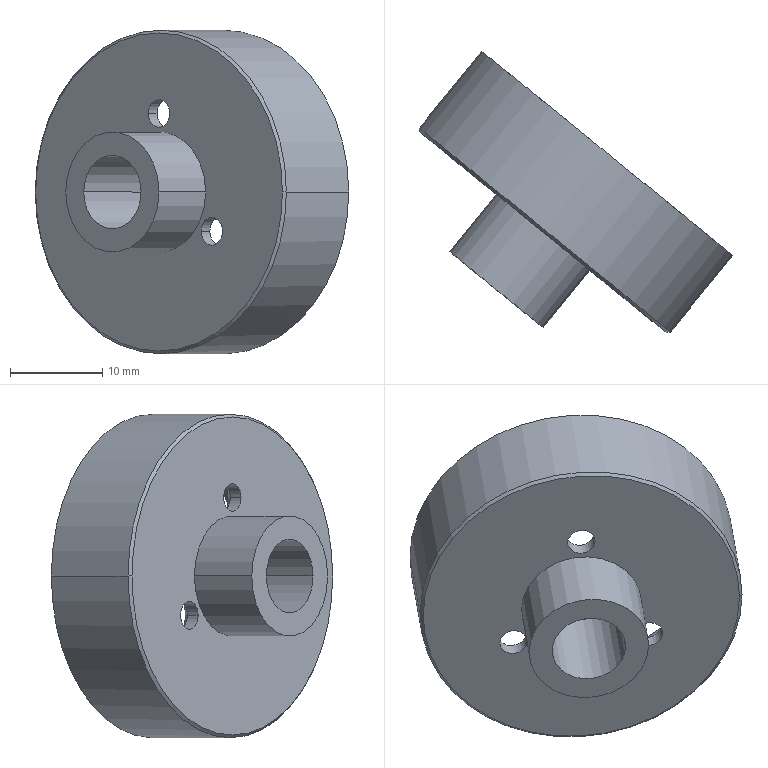Part | SolidWorks | features BaseBody 1 | 1 solid | 29 faces | box 33.905 x 30.428 x 35 mm | volume 5306 mm3 | cylinder 15 | cone 8 | plane 6 | commonest cylinder face diameters 3 x6 30 x3 8 x2 13 x2 35 x2
STEP:
#1=CARTESIAN_POINT('',(530.861,-127.065,299.195));
#2=VERTEX_POINT('',#1);
#3=CARTESIAN_POINT('',(557.55,-148.769,299.195));
#4=VERTEX_POINT('',#3);
#5=CARTESIAN_POINT('',(544.205,-137.917,299.195));
#6=DIRECTION('',(0.6309,0.7758,-0.000000012));
#7=DIRECTION('',(-0.7758,0.6309,0.));
#8=AXIS2_PLACEMENT_3D('',#5,#6,#7);
#9=CIRCLE('',#8,17.2);
#10=EDGE_CURVE('',#2,#4,#9,.T.);
#11=ORIENTED_EDGE('',*,*,#10,.T.);
#12=CARTESIAN_POINT('',(557.972,-148.726,299.195));
#13=VERTEX_POINT('',#12);
#14=CARTESIAN_POINT('',(557.972,-148.726,299.195));
#15=DIRECTION('',(0.9947,0.1025,-0.000000009));
#16=VECTOR('',#15,1000.);
#17=LINE('',#14,#16);
#18=EDGE_CURVE('',#4,#13,#17,.T.);
#19=ORIENTED_EDGE('',*,*,#18,.T.);
#20=CARTESIAN_POINT('',(530.818,-126.643,299.195));
#21=VERTEX_POINT('',#20);
#22=CARTESIAN_POINT('',(544.395,-137.684,299.195));
#23=DIRECTION('',(-0.6309,-0.7758,0.000000012));
#24=DIRECTION('',(-0.08545,0.06949,-0.9939));
#25=AXIS2_PLACEMENT_3D('',#22,#23,#24);
#26=CIRCLE('',#25,17.5);
#27=EDGE_CURVE('',#13,#21,#26,.T.);
#28=ORIENTED_EDGE('',*,*,#27,.T.);
#29=CARTESIAN_POINT('',(530.818,-126.643,299.195));
#30=DIRECTION('',(-0.1025,0.9947,-0.000000009));
#31=VECTOR('',#30,1000.);
#32=LINE('',#29,#31);
#33=EDGE_CURVE('',#2,#21,#32,.T.);
#34=ORIENTED_EDGE('',*,*,#33,.F.);
#35=EDGE_LOOP('',(#11,#19,#28,#34));
#36=FACE_OUTER_BOUND('',#35,.T.);
#37=CARTESIAN_POINT('',(544.395,-137.684,299.195));
#38=DIRECTION('',(0.6309,0.7758,-0.000000012));
#39=DIRECTION('',(-0.7758,0.6309,0.));
#40=AXIS2_PLACEMENT_3D('',#37,#38,#39);
#41=CONICAL_SURFACE('',#40,17.5,0.7854);
#42=ADVANCED_FACE('',(#36),#41,.T.);
#43=CARTESIAN_POINT('',(548.753,-141.615,294.945));
#44=VERTEX_POINT('',#43);
#45=CARTESIAN_POINT('',(551.08,-143.508,294.945));
#46=VERTEX_POINT('',#45);
#47=CARTESIAN_POINT('',(549.917,-142.562,294.945));
#48=DIRECTION('',(-0.6309,-0.7758,0.000000012));
#49=DIRECTION('',(-0.7758,0.6309,0.));
#50=AXIS2_PLACEMENT_3D('',#47,#48,#49);
#51=CIRCLE('',#50,1.5);
#52=EDGE_CURVE('',#44,#46,#51,.T.);
#53=ORIENTED_EDGE('',*,*,#52,.T.);
#54=CARTESIAN_POINT('',(552.027,-142.344,294.945));
#55=VERTEX_POINT('',#54);
#56=CARTESIAN_POINT('',(550.923,-143.702,294.945));
#57=DIRECTION('',(0.6309,0.7758,-0.000000012));
#58=VECTOR('',#57,1000.);
#59=LINE('',#56,#58);
#60=EDGE_CURVE('',#46,#55,#59,.T.);
#61=ORIENTED_EDGE('',*,*,#60,.T.);
#62=CARTESIAN_POINT('',(549.699,-140.451,294.945));
#63=VERTEX_POINT('',#62);
#64=CARTESIAN_POINT('',(550.863,-141.398,294.945));
#65=DIRECTION('',(-0.6309,-0.7758,0.000000012));
#66=DIRECTION('',(-0.7758,0.6309,0.));
#67=AXIS2_PLACEMENT_3D('',#64,#65,#66);
#68=CIRCLE('',#67,1.5);
#69=EDGE_CURVE('',#63,#55,#68,.T.);
#70=ORIENTED_EDGE('',*,*,#69,.F.);
#71=CARTESIAN_POINT('',(548.595,-141.809,294.945));
#72=DIRECTION('',(0.6309,0.7758,-0.000000012));
#73=VECTOR('',#72,1000.);
#74=LINE('',#71,#73);
#75=EDGE_CURVE('',#44,#63,#74,.T.);
#76=ORIENTED_EDGE('',*,*,#75,.F.);
#77=EDGE_LOOP('',(#53,#61,#70,#76));
#78=FACE_OUTER_BOUND('',#77,.T.);
#79=CARTESIAN_POINT('',(549.759,-142.756,294.945));
#80=DIRECTION('',(0.6309,0.7758,-0.000000012));
#81=DIRECTION('',(-0.7758,0.6309,0.));
#82=AXIS2_PLACEMENT_3D('',#79,#80,#81);
#83=CYLINDRICAL_SURFACE('',#82,1.5);
#84=ADVANCED_FACE('',(#78),#83,.F.);
#85=CARTESIAN_POINT('',(543.042,-136.971,307.695));
#86=VERTEX_POINT('',#85);
#87=CARTESIAN_POINT('',(545.369,-138.864,307.695));
#88=VERTEX_POINT('',#87);
#89=CARTESIAN_POINT('',(544.205,-137.917,307.695));
#90=DIRECTION('',(-0.6309,-0.7758,0.000000012));
#91=DIRECTION('',(-0.7758,0.6309,0.));
#92=AXIS2_PLACEMENT_3D('',#89,#90,#91);
#93=CIRCLE('',#92,1.5);
#94=EDGE_CURVE('',#86,#88,#93,.T.);
#95=ORIENTED_EDGE('',*,*,#94,.T.);
#96=CARTESIAN_POINT('',(546.316,-137.7,307.695));
#97=VERTEX_POINT('',#96);
#98=CARTESIAN_POINT('',(545.211,-139.058,307.695));
#99=DIRECTION('',(0.6309,0.7758,-0.000000012));
#100=VECTOR('',#99,1000.);
#101=LINE('',#98,#100);
#102=EDGE_CURVE('',#88,#97,#101,.T.);
#103=ORIENTED_EDGE('',*,*,#102,.T.);
#104=CARTESIAN_POINT('',(543.988,-135.807,307.695));
#105=VERTEX_POINT('',#104);
#106=CARTESIAN_POINT('',(545.152,-136.753,307.695));
#107=DIRECTION('',(-0.6309,-0.7758,0.000000012));
#108=DIRECTION('',(-0.7758,0.6309,0.));
#109=AXIS2_PLACEMENT_3D('',#106,#107,#108);
#110=CIRCLE('',#109,1.5);
#111=EDGE_CURVE('',#105,#97,#110,.T.);
#112=ORIENTED_EDGE('',*,*,#111,.F.);
#113=CARTESIAN_POINT('',(542.884,-137.165,307.695));
#114=DIRECTION('',(0.6309,0.7758,-0.000000012));
#115=VECTOR('',#114,1000.);
#116=LINE('',#113,#115);
#117=EDGE_CURVE('',#86,#105,#116,.T.);
#118=ORIENTED_EDGE('',*,*,#117,.F.);
#119=EDGE_LOOP('',(#95,#103,#112,#118));
#120=FACE_OUTER_BOUND('',#119,.T.);
#121=CARTESIAN_POINT('',(544.048,-138.111,307.695));
#122=DIRECTION('',(0.6309,0.7758,-0.000000012));
#123=DIRECTION('',(-0.7758,0.6309,0.));
#124=AXIS2_PLACEMENT_3D('',#121,#122,#123);
#125=CYLINDRICAL_SURFACE('',#124,1.5);
#126=ADVANCED_FACE('',(#120),#125,.F.);
#127=CARTESIAN_POINT('',(537.331,-132.326,294.945));
#128=VERTEX_POINT('',#127);
#129=CARTESIAN_POINT('',(539.658,-134.219,294.945));
#130=VERTEX_POINT('',#129);
#131=CARTESIAN_POINT('',(538.494,-133.273,294.945));
#132=DIRECTION('',(-0.6309,-0.7758,0.000000012));
#133=DIRECTION('',(-0.7758,0.6309,0.));
#134=AXIS2_PLACEMENT_3D('',#131,#132,#133);
#135=CIRCLE('',#134,1.5);
#136=EDGE_CURVE('',#128,#130,#135,.T.);
#137=ORIENTED_EDGE('',*,*,#136,.T.);
#138=CARTESIAN_POINT('',(540.604,-133.055,294.945));
#139=VERTEX_POINT('',#138);
#140=CARTESIAN_POINT('',(539.5,-134.413,294.945));
#141=DIRECTION('',(0.6309,0.7758,-0.000000012));
#142=VECTOR('',#141,1000.);
#143=LINE('',#140,#142);
#144=EDGE_CURVE('',#130,#139,#143,.T.);
#145=ORIENTED_EDGE('',*,*,#144,.T.);
#146=CARTESIAN_POINT('',(538.277,-131.163,294.945));
#147=VERTEX_POINT('',#146);
#148=CARTESIAN_POINT('',(539.441,-132.109,294.945));
#149=DIRECTION('',(-0.6309,-0.7758,0.000000012));
#150=DIRECTION('',(-0.7758,0.6309,0.));
#151=AXIS2_PLACEMENT_3D('',#148,#149,#150);
#152=CIRCLE('',#151,1.5);
#153=EDGE_CURVE('',#147,#139,#152,.T.);
#154=ORIENTED_EDGE('',*,*,#153,.F.);
#155=CARTESIAN_POINT('',(537.173,-132.52,294.945));
#156=DIRECTION('',(0.6309,0.7758,-0.000000012));
#157=VECTOR('',#156,1000.);
#158=LINE('',#155,#157);
#159=EDGE_CURVE('',#128,#147,#158,.T.);
#160=ORIENTED_EDGE('',*,*,#159,.F.);
#161=EDGE_LOOP('',(#137,#145,#154,#160));
#162=FACE_OUTER_BOUND('',#161,.T.);
#163=CARTESIAN_POINT('',(538.337,-133.467,294.945));
#164=DIRECTION('',(0.6309,0.7758,-0.000000012));
#165=DIRECTION('',(-0.7758,0.6309,0.));
#166=AXIS2_PLACEMENT_3D('',#163,#164,#165);
#167=CYLINDRICAL_SURFACE('',#166,1.5);
#168=ADVANCED_FACE('',(#162),#167,.F.);
#169=CARTESIAN_POINT('',(534.115,-140.023,299.195));
#170=VERTEX_POINT('',#169);
#171=CARTESIAN_POINT('',(544.201,-148.225,299.195));
#172=VERTEX_POINT('',#171);
#173=CARTESIAN_POINT('',(539.158,-144.124,299.195));
#174=DIRECTION('',(0.6309,0.7758,-0.000000012));
#175=DIRECTION('',(-0.7758,0.6309,0.));
#176=AXIS2_PLACEMENT_3D('',#173,#174,#175);
#177=CIRCLE('',#176,6.5);
#178=EDGE_CURVE('',#170,#172,#177,.T.);
#179=ORIENTED_EDGE('',*,*,#178,.T.);
#180=CARTESIAN_POINT('',(549.248,-142.018,299.195));
#181=VERTEX_POINT('',#180);
#182=CARTESIAN_POINT('',(549.248,-142.018,299.195));
#183=DIRECTION('',(0.6309,0.7758,-0.000000012));
#184=VECTOR('',#183,1000.);
#185=LINE('',#182,#184);
#186=EDGE_CURVE('',#172,#181,#185,.T.);
#187=ORIENTED_EDGE('',*,*,#186,.T.);
#188=CARTESIAN_POINT('',(539.162,-133.816,299.195));
#189=VERTEX_POINT('',#188);
#190=CARTESIAN_POINT('',(544.205,-137.917,299.195));
#191=DIRECTION('',(-0.6309,-0.7758,0.000000012));
#192=DIRECTION('',(-0.7758,0.6309,0.));
#193=AXIS2_PLACEMENT_3D('',#190,#191,#192);
#194=CIRCLE('',#193,6.5);
#195=EDGE_CURVE('',#181,#189,#194,.T.);
#196=ORIENTED_EDGE('',*,*,#195,.T.);
#197=CARTESIAN_POINT('',(539.162,-133.816,299.195));
#198=DIRECTION('',(0.6309,0.7758,-0.000000012));
#199=VECTOR('',#198,1000.);
#200=LINE('',#197,#199);
#201=EDGE_CURVE('',#170,#189,#200,.T.);
#202=ORIENTED_EDGE('',*,*,#201,.F.);
#203=EDGE_LOOP('',(#179,#187,#196,#202));
#204=FACE_OUTER_BOUND('',#203,.T.);
#205=CARTESIAN_POINT('',(544.205,-137.917,299.195));
#206=DIRECTION('',(0.6309,0.7758,-0.000000012));
#207=DIRECTION('',(-0.7758,0.6309,0.));
#208=AXIS2_PLACEMENT_3D('',#205,#206,#207);
#209=CYLINDRICAL_SURFACE('',#208,6.5);
#210=ADVANCED_FACE('',(#204),#209,.T.);
#211=CARTESIAN_POINT('',(564.723,-140.424,299.195));
#212=VERTEX_POINT('',#211);
#213=CARTESIAN_POINT('',(537.568,-118.342,299.195));
#214=VERTEX_POINT('',#213);
#215=CARTESIAN_POINT('',(551.146,-129.383,299.195));
#216=DIRECTION('',(-0.6309,-0.7758,0.000000012));
#217=DIRECTION('',(0.7758,-0.6309,0.));
#218=AXIS2_PLACEMENT_3D('',#215,#216,#217);
#219=CIRCLE('',#218,17.5);
#220=EDGE_CURVE('',#212,#214,#219,.T.);
#221=ORIENTED_EDGE('',*,*,#220,.T.);
#222=CARTESIAN_POINT('',(530.628,-126.876,299.195));
#223=DIRECTION('',(-0.6309,-0.7758,0.000000012));
#224=VECTOR('',#223,1000.);
#225=LINE('',#222,#224);
#226=EDGE_CURVE('',#214,#21,#225,.T.);
#227=ORIENTED_EDGE('',*,*,#226,.T.);
#228=ORIENTED_EDGE('',*,*,#27,.F.);
#229=CARTESIAN_POINT('',(557.783,-148.959,299.195));
#230=DIRECTION('',(-0.6309,-0.7758,0.000000012));
#231=VECTOR('',#230,1000.);
#232=LINE('',#229,#231);
#233=EDGE_CURVE('',#212,#13,#232,.T.);
#234=ORIENTED_EDGE('',*,*,#233,.F.);
#235=EDGE_LOOP('',(#221,#227,#228,#234));
#236=FACE_OUTER_BOUND('',#235,.T.);
#237=CARTESIAN_POINT('',(544.205,-137.917,299.195));
#238=DIRECTION('',(-0.6309,-0.7758,0.000000012));
#239=DIRECTION('',(0.7758,-0.6309,0.));
#240=AXIS2_PLACEMENT_3D('',#237,#238,#239);
#241=CYLINDRICAL_SURFACE('',#240,17.5);
#242=ADVANCED_FACE('',(#236),#241,.T.);
#243=ORIENTED_EDGE('',*,*,#69,.T.);
#244=CARTESIAN_POINT('',(554.137,-142.127,294.945));
#245=VERTEX_POINT('',#244);
#246=CARTESIAN_POINT('',(554.137,-142.127,294.945));
#247=DIRECTION('',(0.9947,0.1025,-0.000000009));
#248=VECTOR('',#247,1000.);
#249=LINE('',#246,#248);
#250=EDGE_CURVE('',#55,#245,#249,.T.);
#251=ORIENTED_EDGE('',*,*,#250,.T.);
#252=CARTESIAN_POINT('',(549.482,-138.341,294.945));
#253=VERTEX_POINT('',#252);
#254=CARTESIAN_POINT('',(551.809,-140.234,294.945));
#255=DIRECTION('',(-0.6309,-0.7758,0.000000012));
#256=DIRECTION('',(-0.7758,0.6309,0.));
#257=AXIS2_PLACEMENT_3D('',#254,#255,#256);
#258=CIRCLE('',#257,3.);
#259=EDGE_CURVE('',#253,#245,#258,.T.);
#260=ORIENTED_EDGE('',*,*,#259,.F.);
#261=CARTESIAN_POINT('',(549.482,-138.341,294.945));
#262=DIRECTION('',(-0.1025,0.9947,-0.000000009));
#263=VECTOR('',#262,1000.);
#264=LINE('',#261,#263);
#265=EDGE_CURVE('',#63,#253,#264,.T.);
#266=ORIENTED_EDGE('',*,*,#265,.F.);
#267=EDGE_LOOP('',(#243,#251,#260,#266));
#268=FACE_OUTER_BOUND('',#267,.T.);
#269=CARTESIAN_POINT('',(551.809,-140.234,294.945));
#270=DIRECTION('',(0.6309,0.7758,-0.000000012));
#271=DIRECTION('',(-0.7758,0.6309,0.));
#272=AXIS2_PLACEMENT_3D('',#269,#270,#271);
#273=CONICAL_SURFACE('',#272,3.,0.7854);
#274=ADVANCED_FACE('',(#268),#273,.F.);
#275=ORIENTED_EDGE('',*,*,#111,.T.);
#276=CARTESIAN_POINT('',(548.426,-137.483,307.695));
#277=VERTEX_POINT('',#276);
#278=CARTESIAN_POINT('',(548.426,-137.483,307.695));
#279=DIRECTION('',(0.9947,0.1025,-0.000000009));
#280=VECTOR('',#279,1000.);
#281=LINE('',#278,#280);
#282=EDGE_CURVE('',#97,#277,#281,.T.);
#283=ORIENTED_EDGE('',*,*,#282,.T.);
#284=CARTESIAN_POINT('',(543.771,-133.697,307.695));
#285=VERTEX_POINT('',#284);
#286=CARTESIAN_POINT('',(546.098,-135.59,307.695));
#287=DIRECTION('',(-0.6309,-0.7758,0.000000012));
#288=DIRECTION('',(-0.7758,0.6309,0.));
#289=AXIS2_PLACEMENT_3D('',#286,#287,#288);
#290=CIRCLE('',#289,3.);
#291=EDGE_CURVE('',#285,#277,#290,.T.);
#292=ORIENTED_EDGE('',*,*,#291,.F.);
#293=CARTESIAN_POINT('',(543.771,-133.697,307.695));
#294=DIRECTION('',(-0.1025,0.9947,-0.000000009));
#295=VECTOR('',#294,1000.);
#296=LINE('',#293,#295);
#297=EDGE_CURVE('',#105,#285,#296,.T.);
#298=ORIENTED_EDGE('',*,*,#297,.F.);
#299=EDGE_LOOP('',(#275,#283,#292,#298));
#300=FACE_OUTER_BOUND('',#299,.T.);
#301=CARTESIAN_POINT('',(546.098,-135.59,307.695));
#302=DIRECTION('',(0.6309,0.7758,-0.000000012));
#303=DIRECTION('',(-0.7758,0.6309,0.));
#304=AXIS2_PLACEMENT_3D('',#301,#302,#303);
#305=CONICAL_SURFACE('',#304,3.,0.7854);
#306=ADVANCED_FACE('',(#300),#305,.F.);
#307=ORIENTED_EDGE('',*,*,#153,.T.);
#308=CARTESIAN_POINT('',(542.715,-132.838,294.945));
#309=VERTEX_POINT('',#308);
#310=CARTESIAN_POINT('',(542.715,-132.838,294.945));
#311=DIRECTION('',(0.9947,0.1025,-0.000000009));
#312=VECTOR('',#311,1000.);
#313=LINE('',#310,#312);
#314=EDGE_CURVE('',#139,#309,#313,.T.);
#315=ORIENTED_EDGE('',*,*,#314,.T.);
#316=CARTESIAN_POINT('',(538.06,-129.053,294.945));
#317=VERTEX_POINT('',#316);
#318=CARTESIAN_POINT('',(540.387,-130.945,294.945));
#319=DIRECTION('',(-0.6309,-0.7758,0.000000012));
#320=DIRECTION('',(-0.7758,0.6309,0.));
#321=AXIS2_PLACEMENT_3D('',#318,#319,#320);
#322=CIRCLE('',#321,3.);
#323=EDGE_CURVE('',#317,#309,#322,.T.);
#324=ORIENTED_EDGE('',*,*,#323,.F.);
#325=CARTESIAN_POINT('',(538.06,-129.053,294.945));
#326=DIRECTION('',(-0.1025,0.9947,-0.000000009));
#327=VECTOR('',#326,1000.);
#328=LINE('',#325,#327);
#329=EDGE_CURVE('',#147,#317,#328,.T.);
#330=ORIENTED_EDGE('',*,*,#329,.F.);
#331=EDGE_LOOP('',(#307,#315,#324,#330));
#332=FACE_OUTER_BOUND('',#331,.T.);
#333=CARTESIAN_POINT('',(540.387,-130.945,294.945));
#334=DIRECTION('',(0.6309,0.7758,-0.000000012));
#335=DIRECTION('',(-0.7758,0.6309,0.));
#336=AXIS2_PLACEMENT_3D('',#333,#334,#335);
#337=CONICAL_SURFACE('',#336,3.,0.7854);
#338=ADVANCED_FACE('',(#332),#337,.F.);
#339=CARTESIAN_POINT('',(542.261,-146.648,299.195));
#340=VERTEX_POINT('',#339);
#341=CARTESIAN_POINT('',(536.055,-141.6,299.195));
#342=VERTEX_POINT('',#341);
#343=CARTESIAN_POINT('',(539.158,-144.124,299.195));
#344=DIRECTION('',(0.6309,0.7758,-0.000000012));
#345=DIRECTION('',(-0.7758,0.6309,0.));
#346=AXIS2_PLACEMENT_3D('',#343,#344,#345);
#347=CIRCLE('',#346,4.);
#348=EDGE_CURVE('',#340,#342,#347,.T.);
#349=ORIENTED_EDGE('',*,*,#348,.F.);
#350=CARTESIAN_POINT('',(549.202,-138.113,299.195));
#351=VERTEX_POINT('',#350);
#352=CARTESIAN_POINT('',(549.202,-138.113,299.195));
#353=DIRECTION('',(0.6309,0.7758,-0.000000012));
#354=VECTOR('',#353,1000.);
#355=LINE('',#352,#354);
#356=EDGE_CURVE('',#340,#351,#355,.T.);
#357=ORIENTED_EDGE('',*,*,#356,.T.);
#358=CARTESIAN_POINT('',(542.995,-133.066,299.195));
#359=VERTEX_POINT('',#358);
#360=CARTESIAN_POINT('',(546.098,-135.59,299.195));
#361=DIRECTION('',(0.6309,0.7758,-0.000000012));
#362=DIRECTION('',(-0.7758,0.6309,0.));
#363=AXIS2_PLACEMENT_3D('',#360,#361,#362);
#364=CIRCLE('',#363,4.);
#365=EDGE_CURVE('',#351,#359,#364,.T.);
#366=ORIENTED_EDGE('',*,*,#365,.T.);
#367=CARTESIAN_POINT('',(542.995,-133.066,299.195));
#368=DIRECTION('',(0.6309,0.7758,-0.000000012));
#369=VECTOR('',#368,1000.);
#370=LINE('',#367,#369);
#371=EDGE_CURVE('',#342,#359,#370,.T.);
#372=ORIENTED_EDGE('',*,*,#371,.F.);
#373=EDGE_LOOP('',(#349,#357,#366,#372));
#374=FACE_OUTER_BOUND('',#373,.T.);
#375=CARTESIAN_POINT('',(546.098,-135.59,299.195));
#376=DIRECTION('',(0.6309,0.7758,-0.000000012));
#377=DIRECTION('',(-0.7758,0.6309,0.));
#378=AXIS2_PLACEMENT_3D('',#375,#376,#377);
#379=CYLINDRICAL_SURFACE('',#378,4.);
#380=ADVANCED_FACE('',(#374),#379,.F.);
#381=CARTESIAN_POINT('',(539.508,-119.919,299.195));
#382=VERTEX_POINT('',#381);
#383=CARTESIAN_POINT('',(550.755,-129.066,284.203));
#384=VERTEX_POINT('',#383);
#385=CARTESIAN_POINT('',(551.146,-129.383,299.195));
#386=DIRECTION('',(-0.6309,-0.7758,0.000000012));
#387=DIRECTION('',(0.7758,-0.6309,0.));
#388=AXIS2_PLACEMENT_3D('',#385,#386,#387);
#389=CIRCLE('',#388,15.);
#390=EDGE_CURVE('',#382,#384,#389,.T.);
#391=ORIENTED_EDGE('',*,*,#390,.F.);
#392=CARTESIAN_POINT('',(534.461,-126.126,299.195));
#393=VERTEX_POINT('',#392);
#394=CARTESIAN_POINT('',(539.508,-119.919,299.195));
#395=DIRECTION('',(-0.6309,-0.7758,0.000000012));
#396=VECTOR('',#395,1000.);
#397=LINE('',#394,#396);
#398=EDGE_CURVE('',#382,#393,#397,.T.);
#399=ORIENTED_EDGE('',*,*,#398,.T.);
#400=CARTESIAN_POINT('',(545.708,-135.272,284.203));
#401=VERTEX_POINT('',#400);
#402=CARTESIAN_POINT('',(546.098,-135.59,299.195));
#403=DIRECTION('',(-0.6309,-0.7758,0.000000012));
#404=DIRECTION('',(0.7758,-0.6309,0.));
#405=AXIS2_PLACEMENT_3D('',#402,#403,#404);
#406=CIRCLE('',#405,15.);
#407=EDGE_CURVE('',#393,#401,#406,.T.);
#408=ORIENTED_EDGE('',*,*,#407,.T.);
#409=CARTESIAN_POINT('',(550.755,-129.066,284.203));
#410=DIRECTION('',(0.6309,0.7758,0.));
#411=VECTOR('',#410,1000.);
#412=LINE('',#409,#411);
#413=EDGE_CURVE('',#401,#384,#412,.T.);
#414=ORIENTED_EDGE('',*,*,#413,.T.);
#415=EDGE_LOOP('',(#391,#399,#408,#414));
#416=FACE_OUTER_BOUND('',#415,.T.);
#417=CARTESIAN_POINT('',(551.146,-129.383,299.195));
#418=DIRECTION('',(-0.6309,-0.7758,0.000000012));
#419=DIRECTION('',(0.7758,-0.6309,0.));
#420=AXIS2_PLACEMENT_3D('',#417,#418,#419);
#421=CYLINDRICAL_SURFACE('',#420,15.);
#422=ADVANCED_FACE('',(#416),#421,.F.);
#423=ORIENTED_EDGE('',*,*,#398,.F.);
#424=CARTESIAN_POINT('',(562.783,-138.847,299.195));
#425=VERTEX_POINT('',#424);
#426=CARTESIAN_POINT('',(551.146,-129.383,299.195));
#427=DIRECTION('',(-0.6309,-0.7758,0.000000012));
#428=DIRECTION('',(0.7758,-0.6309,0.));
#429=AXIS2_PLACEMENT_3D('',#426,#427,#428);
#430=CIRCLE('',#429,15.);
#431=EDGE_CURVE('',#425,#382,#430,.T.);
#432=ORIENTED_EDGE('',*,*,#431,.F.);
#433=CARTESIAN_POINT('',(557.736,-145.054,299.195));
#434=VERTEX_POINT('',#433);
#435=CARTESIAN_POINT('',(562.783,-138.847,299.195));
#436=DIRECTION('',(-0.6309,-0.7758,0.000000012));
#437=VECTOR('',#436,1000.);
#438=LINE('',#435,#437);
#439=EDGE_CURVE('',#425,#434,#438,.T.);
#440=ORIENTED_EDGE('',*,*,#439,.T.);
#441=CARTESIAN_POINT('',(546.098,-135.59,299.195));
#442=DIRECTION('',(-0.6309,-0.7758,0.000000012));
#443=DIRECTION('',(0.7758,-0.6309,0.));
#444=AXIS2_PLACEMENT_3D('',#441,#442,#443);
#445=CIRCLE('',#444,15.);
#446=EDGE_CURVE('',#434,#393,#445,.T.);
#447=ORIENTED_EDGE('',*,*,#446,.T.);
#448=EDGE_LOOP('',(#423,#432,#440,#447));
#449=FACE_OUTER_BOUND('',#448,.T.);
#450=CARTESIAN_POINT('',(551.146,-129.383,299.195));
#451=DIRECTION('',(-0.6309,-0.7758,0.000000012));
#452=DIRECTION('',(0.7758,-0.6309,0.));
#453=AXIS2_PLACEMENT_3D('',#450,#451,#452);
#454=CYLINDRICAL_SURFACE('',#453,15.);
#455=ADVANCED_FACE('',(#449),#454,.F.);
#456=ORIENTED_EDGE('',*,*,#10,.F.);
#457=CARTESIAN_POINT('',(544.205,-137.917,299.195));
#458=DIRECTION('',(0.6309,0.7758,-0.000000012));
#459=DIRECTION('',(-0.7758,0.6309,0.));
#460=AXIS2_PLACEMENT_3D('',#457,#458,#459);
#461=CIRCLE('',#460,17.2);
#462=EDGE_CURVE('',#4,#2,#461,.T.);
#463=ORIENTED_EDGE('',*,*,#462,.F.);
#464=EDGE_LOOP('',(#456,#463));
#465=FACE_OUTER_BOUND('',#464,.T.);
#466=ORIENTED_EDGE('',*,*,#52,.F.);
#467=CARTESIAN_POINT('',(549.917,-142.562,294.945));
#468=DIRECTION('',(-0.6309,-0.7758,0.000000012));
#469=DIRECTION('',(-0.7758,0.6309,0.));
#470=AXIS2_PLACEMENT_3D('',#467,#468,#469);
#471=CIRCLE('',#470,1.5);
#472=EDGE_CURVE('',#46,#44,#471,.T.);
#473=ORIENTED_EDGE('',*,*,#472,.F.);
#474=EDGE_LOOP('',(#466,#473));
#475=FACE_BOUND('',#474,.T.);
#476=ORIENTED_EDGE('',*,*,#94,.F.);
#477=CARTESIAN_POINT('',(544.205,-137.917,307.695));
#478=DIRECTION('',(-0.6309,-0.7758,0.000000012));
#479=DIRECTION('',(-0.7758,0.6309,0.));
#480=AXIS2_PLACEMENT_3D('',#477,#478,#479);
#481=CIRCLE('',#480,1.5);
#482=EDGE_CURVE('',#88,#86,#481,.T.);
#483=ORIENTED_EDGE('',*,*,#482,.F.);
#484=EDGE_LOOP('',(#476,#483));
#485=FACE_BOUND('',#484,.T.);
#486=ORIENTED_EDGE('',*,*,#136,.F.);
#487=CARTESIAN_POINT('',(538.494,-133.273,294.945));
#488=DIRECTION('',(-0.6309,-0.7758,0.000000012));
#489=DIRECTION('',(-0.7758,0.6309,0.));
#490=AXIS2_PLACEMENT_3D('',#487,#488,#489);
#491=CIRCLE('',#490,1.5);
#492=EDGE_CURVE('',#130,#128,#491,.T.);
#493=ORIENTED_EDGE('',*,*,#492,.F.);
#494=EDGE_LOOP('',(#486,#493));
#495=FACE_BOUND('',#494,.T.);
#496=CARTESIAN_POINT('',(544.205,-137.917,299.195));
#497=DIRECTION('',(-0.6309,-0.7758,0.000000012));
#498=DIRECTION('',(-0.7758,0.6309,0.));
#499=AXIS2_PLACEMENT_3D('',#496,#497,#498);
#500=CIRCLE('',#499,6.5);
#501=EDGE_CURVE('',#189,#181,#500,.T.);
#502=ORIENTED_EDGE('',*,*,#501,.F.);
#503=ORIENTED_EDGE('',*,*,#195,.F.);
#504=EDGE_LOOP('',(#502,#503));
#505=FACE_BOUND('',#504,.T.);
#506=CARTESIAN_POINT('',(544.205,-137.917,299.195));
#507=DIRECTION('',(0.6309,0.7758,-0.000000012));
#508=DIRECTION('',(-0.7758,0.6309,0.));
#509=AXIS2_PLACEMENT_3D('',#506,#507,#508);
#510=PLANE('',#509);
#511=ADVANCED_FACE('',(#465,#475,#485,#495,#505),#510,.F.);
#512=ORIENTED_EDGE('',*,*,#18,.F.);
#513=ORIENTED_EDGE('',*,*,#462,.T.);
#514=ORIENTED_EDGE('',*,*,#33,.T.);
#515=CARTESIAN_POINT('',(544.395,-137.684,299.195));
#516=DIRECTION('',(-0.6309,-0.7758,0.000000012));
#517=DIRECTION('',(-0.08545,0.06949,-0.9939));
#518=AXIS2_PLACEMENT_3D('',#515,#516,#517);
#519=CIRCLE('',#518,17.5);
#520=EDGE_CURVE('',#21,#13,#519,.T.);
#521=ORIENTED_EDGE('',*,*,#520,.T.);
#522=EDGE_LOOP('',(#512,#513,#514,#521));
#523=FACE_OUTER_BOUND('',#522,.T.);
#524=CARTESIAN_POINT('',(544.395,-137.684,299.195));
#525=DIRECTION('',(0.6309,0.7758,-0.000000012));
#526=DIRECTION('',(-0.7758,0.6309,0.));
#527=AXIS2_PLACEMENT_3D('',#524,#525,#526);
#528=CONICAL_SURFACE('',#527,17.5,0.7854);
#529=ADVANCED_FACE('',(#523),#528,.T.);
#530=ORIENTED_EDGE('',*,*,#60,.F.);
#531=ORIENTED_EDGE('',*,*,#472,.T.);
#532=ORIENTED_EDGE('',*,*,#75,.T.);
#533=CARTESIAN_POINT('',(550.863,-141.398,294.945));
#534=DIRECTION('',(-0.6309,-0.7758,0.000000012));
#535=DIRECTION('',(-0.7758,0.6309,0.));
#536=AXIS2_PLACEMENT_3D('',#533,#534,#535);
#537=CIRCLE('',#536,1.5);
#538=EDGE_CURVE('',#55,#63,#537,.T.);
#539=ORIENTED_EDGE('',*,*,#538,.F.);
#540=EDGE_LOOP('',(#530,#531,#532,#539));
#541=FACE_OUTER_BOUND('',#540,.T.);
#542=CARTESIAN_POINT('',(549.759,-142.756,294.945));
#543=DIRECTION('',(0.6309,0.7758,-0.000000012));
#544=DIRECTION('',(-0.7758,0.6309,0.));
#545=AXIS2_PLACEMENT_3D('',#542,#543,#544);
#546=CYLINDRICAL_SURFACE('',#545,1.5);
#547=ADVANCED_FACE('',(#541),#546,.F.);
#548=ORIENTED_EDGE('',*,*,#102,.F.);
#549=ORIENTED_EDGE('',*,*,#482,.T.);
#550=ORIENTED_EDGE('',*,*,#117,.T.);
#551=CARTESIAN_POINT('',(545.152,-136.753,307.695));
#552=DIRECTION('',(-0.6309,-0.7758,0.000000012));
#553=DIRECTION('',(-0.7758,0.6309,0.));
#554=AXIS2_PLACEMENT_3D('',#551,#552,#553);
#555=CIRCLE('',#554,1.5);
#556=EDGE_CURVE('',#97,#105,#555,.T.);
#557=ORIENTED_EDGE('',*,*,#556,.F.);
#558=EDGE_LOOP('',(#548,#549,#550,#557));
#559=FACE_OUTER_BOUND('',#558,.T.);
#560=CARTESIAN_POINT('',(544.048,-138.111,307.695));
#561=DIRECTION('',(0.6309,0.7758,-0.000000012));
#562=DIRECTION('',(-0.7758,0.6309,0.));
#563=AXIS2_PLACEMENT_3D('',#560,#561,#562);
#564=CYLINDRICAL_SURFACE('',#563,1.5);
#565=ADVANCED_FACE('',(#559),#564,.F.);
#566=ORIENTED_EDGE('',*,*,#144,.F.);
#567=ORIENTED_EDGE('',*,*,#492,.T.);
#568=ORIENTED_EDGE('',*,*,#159,.T.);
#569=CARTESIAN_POINT('',(539.441,-132.109,294.945));
#570=DIRECTION('',(-0.6309,-0.7758,0.000000012));
#571=DIRECTION('',(-0.7758,0.6309,0.));
#572=AXIS2_PLACEMENT_3D('',#569,#570,#571);
#573=CIRCLE('',#572,1.5);
#574=EDGE_CURVE('',#139,#147,#573,.T.);
#575=ORIENTED_EDGE('',*,*,#574,.F.);
#576=EDGE_LOOP('',(#566,#567,#568,#575));
#577=FACE_OUTER_BOUND('',#576,.T.);
#578=CARTESIAN_POINT('',(538.337,-133.467,294.945));
#579=DIRECTION('',(0.6309,0.7758,-0.000000012));
#580=DIRECTION('',(-0.7758,0.6309,0.));
#581=AXIS2_PLACEMENT_3D('',#578,#579,#580);
#582=CYLINDRICAL_SURFACE('',#581,1.5);
#583=ADVANCED_FACE('',(#577),#582,.F.);
#584=ORIENTED_EDGE('',*,*,#186,.F.);
#585=CARTESIAN_POINT('',(539.158,-144.124,299.195));
#586=DIRECTION('',(0.6309,0.7758,-0.000000012));
#587=DIRECTION('',(-0.7758,0.6309,0.));
#588=AXIS2_PLACEMENT_3D('',#585,#586,#587);
#589=CIRCLE('',#588,6.5);
#590=EDGE_CURVE('',#172,#170,#589,.T.);
#591=ORIENTED_EDGE('',*,*,#590,.T.);
#592=ORIENTED_EDGE('',*,*,#201,.T.);
#593=ORIENTED_EDGE('',*,*,#501,.T.);
#594=EDGE_LOOP('',(#584,#591,#592,#593));
#595=FACE_OUTER_BOUND('',#594,.T.);
#596=CARTESIAN_POINT('',(544.205,-137.917,299.195));
#597=DIRECTION('',(0.6309,0.7758,-0.000000012));
#598=DIRECTION('',(-0.7758,0.6309,0.));
#599=AXIS2_PLACEMENT_3D('',#596,#597,#598);
#600=CYLINDRICAL_SURFACE('',#599,6.5);
#601=ADVANCED_FACE('',(#595),#600,.T.);
#602=ORIENTED_EDGE('',*,*,#226,.F.);
#603=CARTESIAN_POINT('',(550.755,-129.066,281.702));
#604=VERTEX_POINT('',#603);
#605=CARTESIAN_POINT('',(551.146,-129.383,299.195));
#606=DIRECTION('',(-0.6309,-0.7758,0.000000012));
#607=DIRECTION('',(0.7758,-0.6309,0.));
#608=AXIS2_PLACEMENT_3D('',#605,#606,#607);
#609=CIRCLE('',#608,17.5);
#610=EDGE_CURVE('',#214,#604,#609,.T.);
#611=ORIENTED_EDGE('',*,*,#610,.T.);
#612=CARTESIAN_POINT('',(545.708,-135.272,281.702));
#613=VERTEX_POINT('',#612);
#614=CARTESIAN_POINT('',(543.815,-137.6,281.702));
#615=DIRECTION('',(-0.6309,-0.7758,0.000000012));
#616=VECTOR('',#615,1000.);
#617=LINE('',#614,#616);
#618=EDGE_CURVE('',#604,#613,#617,.T.);
#619=ORIENTED_EDGE('',*,*,#618,.T.);
#620=CARTESIAN_POINT('',(546.484,-135.903,281.702));
#621=VERTEX_POINT('',#620);
#622=CARTESIAN_POINT('',(546.098,-135.59,299.195));
#623=DIRECTION('',(-0.6309,-0.7758,0.000000012));
#624=DIRECTION('',(0.7758,-0.6309,0.));
#625=AXIS2_PLACEMENT_3D('',#622,#623,#624);
#626=CIRCLE('',#625,17.5);
#627=EDGE_CURVE('',#613,#621,#626,.T.);
#628=ORIENTED_EDGE('',*,*,#627,.T.);
#629=CARTESIAN_POINT('',(551.531,-129.697,281.702));
#630=VERTEX_POINT('',#629);
#631=CARTESIAN_POINT('',(544.591,-138.231,281.702));
#632=DIRECTION('',(0.6309,0.7758,-0.000000012));
#633=VECTOR('',#632,1000.);
#634=LINE('',#631,#633);
#635=EDGE_CURVE('',#621,#630,#634,.T.);
#636=ORIENTED_EDGE('',*,*,#635,.T.);
#637=CARTESIAN_POINT('',(551.146,-129.383,299.195));
#638=DIRECTION('',(-0.6309,-0.7758,0.000000012));
#639=DIRECTION('',(0.7758,-0.6309,0.));
#640=AXIS2_PLACEMENT_3D('',#637,#638,#639);
#641=CIRCLE('',#640,17.5);
#642=EDGE_CURVE('',#630,#212,#641,.T.);
#643=ORIENTED_EDGE('',*,*,#642,.T.);
#644=ORIENTED_EDGE('',*,*,#233,.T.);
#645=ORIENTED_EDGE('',*,*,#520,.F.);
#646=EDGE_LOOP('',(#602,#611,#619,#628,#636,#643,#644,#645));
#647=FACE_OUTER_BOUND('',#646,.T.);
#648=CARTESIAN_POINT('',(544.205,-137.917,299.195));
#649=DIRECTION('',(-0.6309,-0.7758,0.000000012));
#650=DIRECTION('',(0.7758,-0.6309,0.));
#651=AXIS2_PLACEMENT_3D('',#648,#649,#650);
#652=CYLINDRICAL_SURFACE('',#651,17.5);
#653=ADVANCED_FACE('',(#647),#652,.T.);
#654=ORIENTED_EDGE('',*,*,#250,.F.);
#655=ORIENTED_EDGE('',*,*,#538,.T.);
#656=ORIENTED_EDGE('',*,*,#265,.T.);
#657=CARTESIAN_POINT('',(551.809,-140.234,294.945));
#658=DIRECTION('',(-0.6309,-0.7758,0.000000012));
#659=DIRECTION('',(-0.7758,0.6309,0.));
#660=AXIS2_PLACEMENT_3D('',#657,#658,#659);
#661=CIRCLE('',#660,3.);
#662=EDGE_CURVE('',#245,#253,#661,.T.);
#663=ORIENTED_EDGE('',*,*,#662,.F.);
#664=EDGE_LOOP('',(#654,#655,#656,#663));
#665=FACE_OUTER_BOUND('',#664,.T.);
#666=CARTESIAN_POINT('',(551.809,-140.234,294.945));
#667=DIRECTION('',(0.6309,0.7758,-0.000000012));
#668=DIRECTION('',(-0.7758,0.6309,0.));
#669=AXIS2_PLACEMENT_3D('',#666,#667,#668);
#670=CONICAL_SURFACE('',#669,3.,0.7854);
#671=ADVANCED_FACE('',(#665),#670,.F.);
#672=ORIENTED_EDGE('',*,*,#282,.F.);
#673=ORIENTED_EDGE('',*,*,#556,.T.);
#674=ORIENTED_EDGE('',*,*,#297,.T.);
#675=CARTESIAN_POINT('',(546.098,-135.59,307.695));
#676=DIRECTION('',(-0.6309,-0.7758,0.000000012));
#677=DIRECTION('',(-0.7758,0.6309,0.));
#678=AXIS2_PLACEMENT_3D('',#675,#676,#677);
#679=CIRCLE('',#678,3.);
#680=EDGE_CURVE('',#277,#285,#679,.T.);
#681=ORIENTED_EDGE('',*,*,#680,.F.);
#682=EDGE_LOOP('',(#672,#673,#674,#681));
#683=FACE_OUTER_BOUND('',#682,.T.);
#684=CARTESIAN_POINT('',(546.098,-135.59,307.695));
#685=DIRECTION('',(0.6309,0.7758,-0.000000012));
#686=DIRECTION('',(-0.7758,0.6309,0.));
#687=AXIS2_PLACEMENT_3D('',#684,#685,#686);
#688=CONICAL_SURFACE('',#687,3.,0.7854);
#689=ADVANCED_FACE('',(#683),#688,.F.);
#690=ORIENTED_EDGE('',*,*,#314,.F.);
#691=ORIENTED_EDGE('',*,*,#574,.T.);
#692=ORIENTED_EDGE('',*,*,#329,.T.);
#693=CARTESIAN_POINT('',(540.387,-130.945,294.945));
#694=DIRECTION('',(-0.6309,-0.7758,0.000000012));
#695=DIRECTION('',(-0.7758,0.6309,0.));
#696=AXIS2_PLACEMENT_3D('',#693,#694,#695);
#697=CIRCLE('',#696,3.);
#698=EDGE_CURVE('',#309,#317,#697,.T.);
#699=ORIENTED_EDGE('',*,*,#698,.F.);
#700=EDGE_LOOP('',(#690,#691,#692,#699));
#701=FACE_OUTER_BOUND('',#700,.T.);
#702=CARTESIAN_POINT('',(540.387,-130.945,294.945));
#703=DIRECTION('',(0.6309,0.7758,-0.000000012));
#704=DIRECTION('',(-0.7758,0.6309,0.));
#705=AXIS2_PLACEMENT_3D('',#702,#703,#704);
#706=CONICAL_SURFACE('',#705,3.,0.7854);
#707=ADVANCED_FACE('',(#701),#706,.F.);
#708=ORIENTED_EDGE('',*,*,#178,.F.);
#709=ORIENTED_EDGE('',*,*,#590,.F.);
#710=EDGE_LOOP('',(#708,#709));
#711=FACE_OUTER_BOUND('',#710,.T.);
#712=CARTESIAN_POINT('',(539.158,-144.124,299.195));
#713=DIRECTION('',(0.6309,0.7758,-0.000000012));
#714=DIRECTION('',(-0.7758,0.6309,0.));
#715=AXIS2_PLACEMENT_3D('',#712,#713,#714);
#716=CIRCLE('',#715,4.);
#717=EDGE_CURVE('',#342,#340,#716,.T.);
#718=ORIENTED_EDGE('',*,*,#717,.T.);
#719=ORIENTED_EDGE('',*,*,#348,.T.);
#720=EDGE_LOOP('',(#718,#719));
#721=FACE_BOUND('',#720,.T.);
#722=CARTESIAN_POINT('',(539.158,-144.124,299.195));
#723=DIRECTION('',(-0.6309,-0.7758,0.000000012));
#724=DIRECTION('',(0.7758,-0.6309,0.));
#725=AXIS2_PLACEMENT_3D('',#722,#723,#724);
#726=PLANE('',#725);
#727=ADVANCED_FACE('',(#711,#721),#726,.T.);
#728=CARTESIAN_POINT('',(551.531,-129.697,284.203));
#729=VERTEX_POINT('',#728);
#730=CARTESIAN_POINT('',(551.146,-129.383,299.195));
#731=DIRECTION('',(-0.6309,-0.7758,0.000000012));
#732=DIRECTION('',(0.7758,-0.6309,0.));
#733=AXIS2_PLACEMENT_3D('',#730,#731,#732);
#734=CIRCLE('',#733,15.);
#735=EDGE_CURVE('',#729,#425,#734,.T.);
#736=ORIENTED_EDGE('',*,*,#735,.T.);
#737=ORIENTED_EDGE('',*,*,#431,.T.);
#738=ORIENTED_EDGE('',*,*,#390,.T.);
#739=CARTESIAN_POINT('',(550.755,-129.066,299.195));
#740=DIRECTION('',(-0.000000008,-0.000000009,-1.));
#741=VECTOR('',#740,1000.);
#742=LINE('',#739,#741);
#743=EDGE_CURVE('',#384,#604,#742,.T.);
#744=ORIENTED_EDGE('',*,*,#743,.T.);
#745=ORIENTED_EDGE('',*,*,#610,.F.);
#746=ORIENTED_EDGE('',*,*,#220,.F.);
#747=ORIENTED_EDGE('',*,*,#642,.F.);
#748=CARTESIAN_POINT('',(551.531,-129.697,299.195));
#749=DIRECTION('',(0.000000008,0.000000009,1.));
#750=VECTOR('',#749,1000.);
#751=LINE('',#748,#750);
#752=EDGE_CURVE('',#630,#729,#751,.T.);
#753=ORIENTED_EDGE('',*,*,#752,.T.);
#754=EDGE_LOOP('',(#736,#737,#738,#744,#745,#746,#747,#753));
#755=FACE_OUTER_BOUND('',#754,.T.);
#756=CARTESIAN_POINT('',(551.146,-129.383,299.195));
#757=DIRECTION('',(0.6309,0.7758,-0.000000012));
#758=DIRECTION('',(-0.7758,0.6309,0.));
#759=AXIS2_PLACEMENT_3D('',#756,#757,#758);
#760=PLANE('',#759);
#761=ADVANCED_FACE('',(#755),#760,.T.);
#762=ORIENTED_EDGE('',*,*,#752,.F.);
#763=ORIENTED_EDGE('',*,*,#635,.F.);
#764=CARTESIAN_POINT('',(546.484,-135.903,284.203));
#765=VERTEX_POINT('',#764);
#766=CARTESIAN_POINT('',(546.484,-135.903,287.719));
#767=DIRECTION('',(-0.000000016,0.000000013,-1.));
#768=VECTOR('',#767,1000.);
#769=LINE('',#766,#768);
#770=EDGE_CURVE('',#765,#621,#769,.T.);
#771=ORIENTED_EDGE('',*,*,#770,.F.);
#772=CARTESIAN_POINT('',(551.531,-129.697,284.203));
#773=DIRECTION('',(-0.6309,-0.7758,0.));
#774=VECTOR('',#773,1000.);
#775=LINE('',#772,#774);
#776=EDGE_CURVE('',#729,#765,#775,.T.);
#777=ORIENTED_EDGE('',*,*,#776,.F.);
#778=EDGE_LOOP('',(#762,#763,#771,#777));
#779=FACE_OUTER_BOUND('',#778,.T.);
#780=CARTESIAN_POINT('',(551.531,-129.697,287.719));
#781=DIRECTION('',(0.7758,-0.6309,-0.000000021));
#782=DIRECTION('',(0.6309,0.7758,0.));
#783=AXIS2_PLACEMENT_3D('',#780,#781,#782);
#784=PLANE('',#783);
#785=ADVANCED_FACE('',(#779),#784,.F.);
#786=CARTESIAN_POINT('',(545.708,-135.272,279.776));
#787=DIRECTION('',(0.000000016,-0.000000013,1.));
#788=VECTOR('',#787,1000.);
#789=LINE('',#786,#788);
#790=EDGE_CURVE('',#613,#401,#789,.T.);
#791=ORIENTED_EDGE('',*,*,#790,.F.);
#792=ORIENTED_EDGE('',*,*,#618,.F.);
#793=ORIENTED_EDGE('',*,*,#743,.F.);
#794=ORIENTED_EDGE('',*,*,#413,.F.);
#795=EDGE_LOOP('',(#791,#792,#793,#794));
#796=FACE_OUTER_BOUND('',#795,.T.);
#797=CARTESIAN_POINT('',(550.755,-129.066,279.776));
#798=DIRECTION('',(-0.7758,0.6309,0.000000021));
#799=DIRECTION('',(-0.6309,-0.7758,0.));
#800=AXIS2_PLACEMENT_3D('',#797,#798,#799);
#801=PLANE('',#800);
#802=ADVANCED_FACE('',(#796),#801,.F.);
#803=CARTESIAN_POINT('',(546.098,-135.59,299.195));
#804=DIRECTION('',(-0.6309,-0.7758,0.000000012));
#805=DIRECTION('',(0.7758,-0.6309,0.));
#806=AXIS2_PLACEMENT_3D('',#803,#804,#805);
#807=CIRCLE('',#806,15.);
#808=EDGE_CURVE('',#765,#434,#807,.T.);
#809=ORIENTED_EDGE('',*,*,#808,.F.);
#810=ORIENTED_EDGE('',*,*,#770,.T.);
#811=ORIENTED_EDGE('',*,*,#627,.F.);
#812=ORIENTED_EDGE('',*,*,#790,.T.);
#813=ORIENTED_EDGE('',*,*,#407,.F.);
#814=ORIENTED_EDGE('',*,*,#446,.F.);
#815=EDGE_LOOP('',(#809,#810,#811,#812,#813,#814));
#816=FACE_OUTER_BOUND('',#815,.T.);
#817=ORIENTED_EDGE('',*,*,#259,.T.);
#818=ORIENTED_EDGE('',*,*,#662,.T.);
#819=EDGE_LOOP('',(#817,#818));
#820=FACE_BOUND('',#819,.T.);
#821=ORIENTED_EDGE('',*,*,#291,.T.);
#822=ORIENTED_EDGE('',*,*,#680,.T.);
#823=EDGE_LOOP('',(#821,#822));
#824=FACE_BOUND('',#823,.T.);
#825=ORIENTED_EDGE('',*,*,#323,.T.);
#826=ORIENTED_EDGE('',*,*,#698,.T.);
#827=EDGE_LOOP('',(#825,#826));
#828=FACE_BOUND('',#827,.T.);
#829=CARTESIAN_POINT('',(546.098,-135.59,299.195));
#830=DIRECTION('',(0.6309,0.7758,-0.000000012));
#831=DIRECTION('',(-0.7758,0.6309,0.));
#832=AXIS2_PLACEMENT_3D('',#829,#830,#831);
#833=CIRCLE('',#832,4.);
#834=EDGE_CURVE('',#359,#351,#833,.T.);
#835=ORIENTED_EDGE('',*,*,#834,.F.);
#836=ORIENTED_EDGE('',*,*,#365,.F.);
#837=EDGE_LOOP('',(#835,#836));
#838=FACE_BOUND('',#837,.T.);
#839=CARTESIAN_POINT('',(546.098,-135.59,299.195));
#840=DIRECTION('',(-0.6309,-0.7758,0.000000012));
#841=DIRECTION('',(0.7758,-0.6309,0.));
#842=AXIS2_PLACEMENT_3D('',#839,#840,#841);
#843=PLANE('',#842);
#844=ADVANCED_FACE('',(#816,#820,#824,#828,#838),#843,.F.);
#845=ORIENTED_EDGE('',*,*,#356,.F.);
#846=ORIENTED_EDGE('',*,*,#717,.F.);
#847=ORIENTED_EDGE('',*,*,#371,.T.);
#848=ORIENTED_EDGE('',*,*,#834,.T.);
#849=EDGE_LOOP('',(#845,#846,#847,#848));
#850=FACE_OUTER_BOUND('',#849,.T.);
#851=CARTESIAN_POINT('',(546.098,-135.59,299.195));
#852=DIRECTION('',(0.6309,0.7758,-0.000000012));
#853=DIRECTION('',(-0.7758,0.6309,0.));
#854=AXIS2_PLACEMENT_3D('',#851,#852,#853);
#855=CYLINDRICAL_SURFACE('',#854,4.);
#856=ADVANCED_FACE('',(#850),#855,.F.);
#857=ORIENTED_EDGE('',*,*,#439,.F.);
#858=ORIENTED_EDGE('',*,*,#735,.F.);
#859=ORIENTED_EDGE('',*,*,#776,.T.);
#860=ORIENTED_EDGE('',*,*,#808,.T.);
#861=EDGE_LOOP('',(#857,#858,#859,#860));
#862=FACE_OUTER_BOUND('',#861,.T.);
#863=CARTESIAN_POINT('',(551.146,-129.383,299.195));
#864=DIRECTION('',(-0.6309,-0.7758,0.000000012));
#865=DIRECTION('',(0.7758,-0.6309,0.));
#866=AXIS2_PLACEMENT_3D('',#863,#864,#865);
#867=CYLINDRICAL_SURFACE('',#866,15.);
#868=ADVANCED_FACE('',(#862),#867,.F.);
#869=CLOSED_SHELL('',(#42,#84,#126,#168,#210,#242,#274,#306,#338,#380,#422,#455,#511,#529,#547,#565,#583,#601,#653,#671,#689,#707,#727,#761,#785,#802,#844,#856,#868));
#870=MANIFOLD_SOLID_BREP('',#869);
#871=CARTESIAN_POINT('',(0.,0.,0.));
#872=DIRECTION('',(0.,0.,1.));
#873=DIRECTION('',(1.,0.,0.));
#874=AXIS2_PLACEMENT_3D('',#871,#872,#873);
#875=(LENGTH_UNIT()NAMED_UNIT(*)SI_UNIT(.MILLI.,.METRE.));
#876=UNCERTAINTY_MEASURE_WITH_UNIT(LENGTH_MEASURE(0.00001),#875,'','');
#877=(NAMED_UNIT(*)PLANE_ANGLE_UNIT()SI_UNIT($,.RADIAN.));
#878=(NAMED_UNIT(*)SI_UNIT($,.STERADIAN.)SOLID_ANGLE_UNIT());
#879=(GEOMETRIC_REPRESENTATION_CONTEXT(3)GLOBAL_UNCERTAINTY_ASSIGNED_CONTEXT((#876))GLOBAL_UNIT_ASSIGNED_CONTEXT((#875,#877,#878))REPRESENTATION_CONTEXT('',''));
#880=ADVANCED_BREP_SHAPE_REPRESENTATION('',(#870,#874),#879);